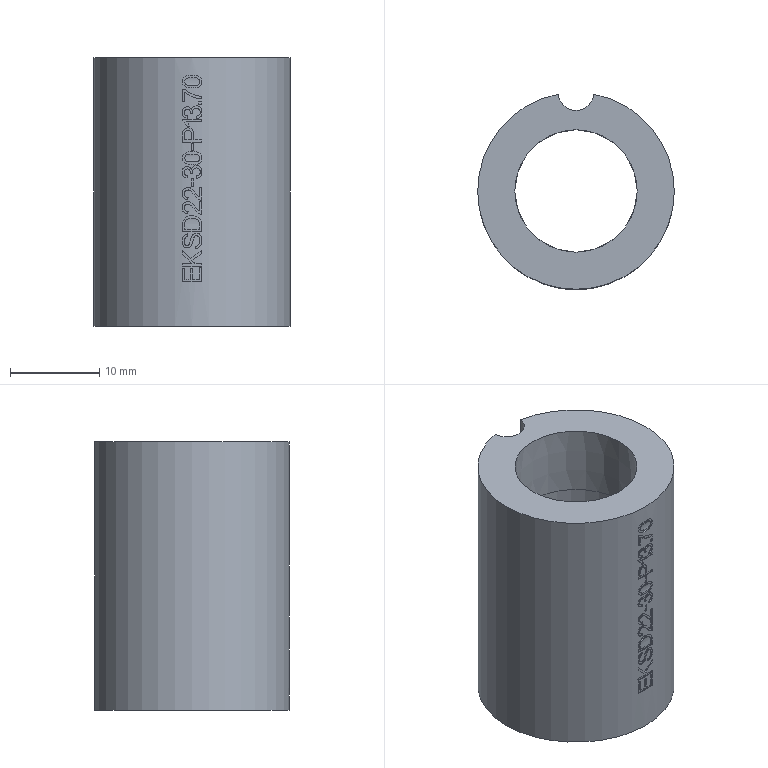Part | NX | features EKSD22-30-P13.70_2 2 | 1 solid | 199 faces | box 22 x 21.819 x 30 mm | volume 6354 mm3 | plane 112 | cylinder 86 | cone 1 | commonest cylinder face diameters 21.8 x16 22 x5 1.281 x4 0.752 x2 0.832 x2 0.882 x2